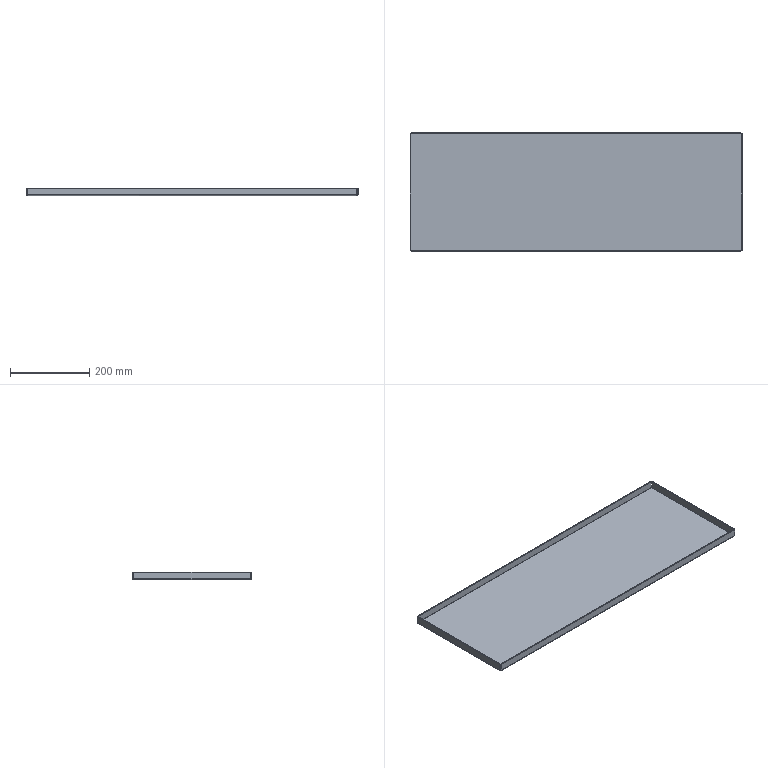Part | STEP file | Part 14 | 1 solid | 38 faces | box 840 x 300 x 20 mm | volume 582338 mm3 | plane 22 | spline 8 | cylinder 8 | commonest cylinder face diameters 1 x4 5 x4
STEP:
#1=CARTESIAN_POINT('',(-417.5,-147.5,-2.));
#2=VERTEX_POINT('',#1);
#3=CARTESIAN_POINT('',(-417.5,147.5,-2.));
#4=VERTEX_POINT('',#3);
#5=CARTESIAN_POINT('',(-417.5,-147.5,-2.));
#6=DIRECTION('',(0.,1.,0.));
#7=VECTOR('',#6,1000.);
#8=LINE('',#5,#7);
#9=EDGE_CURVE('',#2,#4,#8,.T.);
#10=ORIENTED_EDGE('',*,*,#9,.T.);
#11=CARTESIAN_POINT('',(417.5,147.5,-2.));
#12=VERTEX_POINT('',#11);
#13=CARTESIAN_POINT('',(-417.5,147.5,-2.));
#14=DIRECTION('',(1.,0.,0.));
#15=VECTOR('',#14,1000.);
#16=LINE('',#13,#15);
#17=EDGE_CURVE('',#4,#12,#16,.T.);
#18=ORIENTED_EDGE('',*,*,#17,.T.);
#19=CARTESIAN_POINT('',(417.5,-147.5,-2.));
#20=VERTEX_POINT('',#19);
#21=CARTESIAN_POINT('',(417.5,147.5,-2.));
#22=DIRECTION('',(0.,-1.,0.));
#23=VECTOR('',#22,1000.);
#24=LINE('',#21,#23);
#25=EDGE_CURVE('',#12,#20,#24,.T.);
#26=ORIENTED_EDGE('',*,*,#25,.T.);
#27=CARTESIAN_POINT('',(417.5,-147.5,-2.));
#28=DIRECTION('',(-1.,0.,0.));
#29=VECTOR('',#28,1000.);
#30=LINE('',#27,#29);
#31=EDGE_CURVE('',#20,#2,#30,.T.);
#32=ORIENTED_EDGE('',*,*,#31,.T.);
#33=EDGE_LOOP('',(#10,#18,#26,#32));
#34=FACE_OUTER_BOUND('',#33,.T.);
#35=CARTESIAN_POINT('',(0.,0.,-2.));
#36=DIRECTION('',(0.,0.,1.));
#37=DIRECTION('',(1.,0.,0.));
#38=AXIS2_PLACEMENT_3D('',#35,#36,#37);
#39=PLANE('',#38);
#40=ADVANCED_FACE('',(#34),#39,.F.);
#41=CARTESIAN_POINT('',(-417.5,147.5,0.));
#42=VERTEX_POINT('',#41);
#43=CARTESIAN_POINT('',(417.5,147.5,0.));
#44=VERTEX_POINT('',#43);
#45=CARTESIAN_POINT('',(-417.5,147.5,0.));
#46=DIRECTION('',(1.,0.,0.));
#47=VECTOR('',#46,1000.);
#48=LINE('',#45,#47);
#49=EDGE_CURVE('',#42,#44,#48,.T.);
#50=ORIENTED_EDGE('',*,*,#49,.F.);
#51=CARTESIAN_POINT('',(-417.5,-147.5,0.));
#52=VERTEX_POINT('',#51);
#53=CARTESIAN_POINT('',(-417.5,-147.5,0.));
#54=DIRECTION('',(0.,1.,0.));
#55=VECTOR('',#54,1000.);
#56=LINE('',#53,#55);
#57=EDGE_CURVE('',#52,#42,#56,.T.);
#58=ORIENTED_EDGE('',*,*,#57,.F.);
#59=CARTESIAN_POINT('',(417.5,-147.5,0.));
#60=VERTEX_POINT('',#59);
#61=CARTESIAN_POINT('',(417.5,-147.5,0.));
#62=DIRECTION('',(-1.,0.,0.));
#63=VECTOR('',#62,1000.);
#64=LINE('',#61,#63);
#65=EDGE_CURVE('',#60,#52,#64,.T.);
#66=ORIENTED_EDGE('',*,*,#65,.F.);
#67=CARTESIAN_POINT('',(417.5,147.5,0.));
#68=DIRECTION('',(0.,-1.,0.));
#69=VECTOR('',#68,1000.);
#70=LINE('',#67,#69);
#71=EDGE_CURVE('',#44,#60,#70,.T.);
#72=ORIENTED_EDGE('',*,*,#71,.F.);
#73=EDGE_LOOP('',(#50,#58,#66,#72));
#74=FACE_OUTER_BOUND('',#73,.T.);
#75=CARTESIAN_POINT('',(0.,0.,0.));
#76=DIRECTION('',(0.,0.,1.));
#77=DIRECTION('',(1.,0.,0.));
#78=AXIS2_PLACEMENT_3D('',#75,#76,#77);
#79=PLANE('',#78);
#80=ADVANCED_FACE('',(#74),#79,.T.);
#81=CARTESIAN_POINT('',(417.293,150.,0.5));
#82=VERTEX_POINT('',#81);
#83=CARTESIAN_POINT('',(417.293,148.,0.5));
#84=VERTEX_POINT('',#83);
#85=CARTESIAN_POINT('',(417.293,148.,0.5));
#86=DIRECTION('',(0.,-1.,0.));
#87=VECTOR('',#86,1000.);
#88=LINE('',#85,#87);
#89=EDGE_CURVE('',#82,#84,#88,.T.);
#90=ORIENTED_EDGE('',*,*,#89,.T.);
#91=CARTESIAN_POINT('',(417.5,147.5,0.));
#92=CARTESIAN_POINT('',(417.465,147.631,0.));
#93=CARTESIAN_POINT('',(417.431,147.761,0.05389));
#94=CARTESIAN_POINT('',(417.362,147.946,0.239));
#95=CARTESIAN_POINT('',(417.327,148.,0.3691));
#96=CARTESIAN_POINT('',(417.293,148.,0.5));
#97=B_SPLINE_CURVE_WITH_KNOTS('',3,(#91,#92,#93,#94,#95,#96),.UNSPECIFIED.,.F.,.F.,(4,2,4),(0.,0.5,1.),.UNSPECIFIED.);
#98=EDGE_CURVE('',#44,#84,#97,.T.);
#99=ORIENTED_EDGE('',*,*,#98,.F.);
#100=CARTESIAN_POINT('',(417.5,147.5,0.));
#101=DIRECTION('',(0.,0.,-1.));
#102=VECTOR('',#101,1000.);
#103=LINE('',#100,#102);
#104=EDGE_CURVE('',#44,#12,#103,.T.);
#105=ORIENTED_EDGE('',*,*,#104,.T.);
#106=CARTESIAN_POINT('',(417.5,147.5,-2.));
#107=CARTESIAN_POINT('',(417.483,147.827,-2.));
#108=CARTESIAN_POINT('',(417.465,148.154,-1.935));
#109=CARTESIAN_POINT('',(417.431,148.759,-1.684));
#110=CARTESIAN_POINT('',(417.414,149.036,-1.499));
#111=CARTESIAN_POINT('',(417.379,149.499,-1.036));
#112=CARTESIAN_POINT('',(417.362,149.684,-0.759));
#113=CARTESIAN_POINT('',(417.327,149.935,-0.1544));
#114=CARTESIAN_POINT('',(417.31,150.,0.1728));
#115=CARTESIAN_POINT('',(417.293,150.,0.5));
#116=B_SPLINE_CURVE_WITH_KNOTS('',3,(#106,#107,#108,#109,#110,#111,#112,#113,#114,#115),.UNSPECIFIED.,.F.,.F.,(4,2,2,2,4),(0.,0.25,0.5,0.75,1.),.UNSPECIFIED.);
#117=EDGE_CURVE('',#12,#82,#116,.T.);
#118=ORIENTED_EDGE('',*,*,#117,.T.);
#119=EDGE_LOOP('',(#90,#99,#105,#118));
#120=FACE_OUTER_BOUND('',#119,.T.);
#121=CARTESIAN_POINT('',(417.5,147.5,-2.02));
#122=CARTESIAN_POINT('',(417.483,147.83,-2.02));
#123=CARTESIAN_POINT('',(417.465,148.16,-1.954));
#124=CARTESIAN_POINT('',(417.431,148.769,-1.702));
#125=CARTESIAN_POINT('',(417.414,149.049,-1.515));
#126=CARTESIAN_POINT('',(417.379,149.515,-1.049));
#127=CARTESIAN_POINT('',(417.362,149.702,-0.7691));
#128=CARTESIAN_POINT('',(417.327,149.954,-0.1596));
#129=CARTESIAN_POINT('',(417.31,150.02,0.1701));
#130=CARTESIAN_POINT('',(417.293,150.02,0.5));
#131=CARTESIAN_POINT('',(417.5,147.5,-2.));
#132=CARTESIAN_POINT('',(417.483,147.827,-2.));
#133=CARTESIAN_POINT('',(417.465,148.154,-1.935));
#134=CARTESIAN_POINT('',(417.431,148.759,-1.684));
#135=CARTESIAN_POINT('',(417.414,149.036,-1.499));
#136=CARTESIAN_POINT('',(417.379,149.499,-1.036));
#137=CARTESIAN_POINT('',(417.362,149.684,-0.759));
#138=CARTESIAN_POINT('',(417.327,149.935,-0.1544));
#139=CARTESIAN_POINT('',(417.31,150.,0.1727));
#140=CARTESIAN_POINT('',(417.293,150.,0.5));
#141=CARTESIAN_POINT('',(417.5,147.5,0.));
#142=CARTESIAN_POINT('',(417.483,147.565,0.));
#143=CARTESIAN_POINT('',(417.465,147.631,0.01301));
#144=CARTESIAN_POINT('',(417.431,147.752,0.06311));
#145=CARTESIAN_POINT('',(417.414,147.807,0.1002));
#146=CARTESIAN_POINT('',(417.379,147.9,0.1927));
#147=CARTESIAN_POINT('',(417.362,147.937,0.2482));
#148=CARTESIAN_POINT('',(417.327,147.987,0.3691));
#149=CARTESIAN_POINT('',(417.31,148.,0.4345));
#150=CARTESIAN_POINT('',(417.293,148.,0.5));
#151=CARTESIAN_POINT('',(417.5,147.5,0.0202));
#152=CARTESIAN_POINT('',(417.483,147.563,0.0202));
#153=CARTESIAN_POINT('',(417.465,147.626,0.03269));
#154=CARTESIAN_POINT('',(417.431,147.742,0.08076));
#155=CARTESIAN_POINT('',(417.414,147.795,0.1163));
#156=CARTESIAN_POINT('',(417.379,147.884,0.2051));
#157=CARTESIAN_POINT('',(417.362,147.919,0.2584));
#158=CARTESIAN_POINT('',(417.327,147.967,0.3744));
#159=CARTESIAN_POINT('',(417.31,147.98,0.4372));
#160=CARTESIAN_POINT('',(417.293,147.98,0.5));
#161=B_SPLINE_SURFACE_WITH_KNOTS('',1,3,((#121,#122,#123,#124,#125,#126,#127,#128,#129,#130),(#131,#132,#133,#134,#135,#136,#137,#138,#139,#140),(#141,#142,#143,#144,#145,#146,#147,#148,#149,#150),(#151,#152,#153,#154,#155,#156,#157,#158,#159,#160)),.UNSPECIFIED.,.F.,.F.,.F.,(2,1,1,2),(4,2,2,2,4),(-0.01,0.,1.,1.01),(0.,0.25,0.5,0.75,1.),.UNSPECIFIED.);
#162=ADVANCED_FACE('',(#120),#161,.F.);
#163=CARTESIAN_POINT('',(-417.293,148.,0.5));
#164=VERTEX_POINT('',#163);
#165=CARTESIAN_POINT('',(-417.293,148.,0.5));
#166=CARTESIAN_POINT('',(-417.327,148.,0.3691));
#167=CARTESIAN_POINT('',(-417.362,147.946,0.239));
#168=CARTESIAN_POINT('',(-417.431,147.761,0.05389));
#169=CARTESIAN_POINT('',(-417.465,147.631,0.));
#170=CARTESIAN_POINT('',(-417.5,147.5,0.));
#171=B_SPLINE_CURVE_WITH_KNOTS('',3,(#165,#166,#167,#168,#169,#170),.UNSPECIFIED.,.F.,.F.,(4,2,4),(0.,0.5,1.),.UNSPECIFIED.);
#172=EDGE_CURVE('',#164,#42,#171,.T.);
#173=ORIENTED_EDGE('',*,*,#172,.F.);
#174=CARTESIAN_POINT('',(-417.293,150.,0.5));
#175=VERTEX_POINT('',#174);
#176=CARTESIAN_POINT('',(-417.293,148.,0.5));
#177=DIRECTION('',(0.,-1.,0.));
#178=VECTOR('',#177,1000.);
#179=LINE('',#176,#178);
#180=EDGE_CURVE('',#175,#164,#179,.T.);
#181=ORIENTED_EDGE('',*,*,#180,.F.);
#182=CARTESIAN_POINT('',(-417.293,150.,0.5));
#183=CARTESIAN_POINT('',(-417.31,150.,0.1728));
#184=CARTESIAN_POINT('',(-417.327,149.935,-0.1544));
#185=CARTESIAN_POINT('',(-417.362,149.684,-0.759));
#186=CARTESIAN_POINT('',(-417.379,149.499,-1.036));
#187=CARTESIAN_POINT('',(-417.414,149.036,-1.499));
#188=CARTESIAN_POINT('',(-417.431,148.759,-1.684));
#189=CARTESIAN_POINT('',(-417.465,148.154,-1.935));
#190=CARTESIAN_POINT('',(-417.483,147.827,-2.));
#191=CARTESIAN_POINT('',(-417.5,147.5,-2.));
#192=B_SPLINE_CURVE_WITH_KNOTS('',3,(#182,#183,#184,#185,#186,#187,#188,#189,#190,#191),.UNSPECIFIED.,.F.,.F.,(4,2,2,2,4),(0.,0.25,0.5,0.75,1.),.UNSPECIFIED.);
#193=EDGE_CURVE('',#175,#4,#192,.T.);
#194=ORIENTED_EDGE('',*,*,#193,.T.);
#195=CARTESIAN_POINT('',(-417.5,147.5,0.));
#196=DIRECTION('',(0.,0.,-1.));
#197=VECTOR('',#196,1000.);
#198=LINE('',#195,#197);
#199=EDGE_CURVE('',#42,#4,#198,.T.);
#200=ORIENTED_EDGE('',*,*,#199,.F.);
#201=EDGE_LOOP('',(#173,#181,#194,#200));
#202=FACE_OUTER_BOUND('',#201,.T.);
#203=CARTESIAN_POINT('',(-417.293,150.02,0.5));
#204=CARTESIAN_POINT('',(-417.31,150.02,0.1701));
#205=CARTESIAN_POINT('',(-417.327,149.954,-0.1596));
#206=CARTESIAN_POINT('',(-417.362,149.702,-0.7691));
#207=CARTESIAN_POINT('',(-417.379,149.515,-1.049));
#208=CARTESIAN_POINT('',(-417.414,149.049,-1.515));
#209=CARTESIAN_POINT('',(-417.431,148.769,-1.702));
#210=CARTESIAN_POINT('',(-417.465,148.16,-1.954));
#211=CARTESIAN_POINT('',(-417.483,147.83,-2.02));
#212=CARTESIAN_POINT('',(-417.5,147.5,-2.02));
#213=CARTESIAN_POINT('',(-417.293,150.,0.5));
#214=CARTESIAN_POINT('',(-417.31,150.,0.1727));
#215=CARTESIAN_POINT('',(-417.327,149.935,-0.1544));
#216=CARTESIAN_POINT('',(-417.362,149.684,-0.759));
#217=CARTESIAN_POINT('',(-417.379,149.499,-1.036));
#218=CARTESIAN_POINT('',(-417.414,149.036,-1.499));
#219=CARTESIAN_POINT('',(-417.431,148.759,-1.684));
#220=CARTESIAN_POINT('',(-417.465,148.154,-1.935));
#221=CARTESIAN_POINT('',(-417.483,147.827,-2.));
#222=CARTESIAN_POINT('',(-417.5,147.5,-2.));
#223=CARTESIAN_POINT('',(-417.293,148.,0.5));
#224=CARTESIAN_POINT('',(-417.31,148.,0.4345));
#225=CARTESIAN_POINT('',(-417.327,147.987,0.3691));
#226=CARTESIAN_POINT('',(-417.362,147.937,0.2482));
#227=CARTESIAN_POINT('',(-417.379,147.9,0.1927));
#228=CARTESIAN_POINT('',(-417.414,147.807,0.1002));
#229=CARTESIAN_POINT('',(-417.431,147.752,0.06311));
#230=CARTESIAN_POINT('',(-417.465,147.631,0.01301));
#231=CARTESIAN_POINT('',(-417.483,147.565,0.));
#232=CARTESIAN_POINT('',(-417.5,147.5,0.));
#233=CARTESIAN_POINT('',(-417.293,147.98,0.5));
#234=CARTESIAN_POINT('',(-417.31,147.98,0.4372));
#235=CARTESIAN_POINT('',(-417.327,147.967,0.3744));
#236=CARTESIAN_POINT('',(-417.362,147.919,0.2584));
#237=CARTESIAN_POINT('',(-417.379,147.884,0.2051));
#238=CARTESIAN_POINT('',(-417.414,147.795,0.1163));
#239=CARTESIAN_POINT('',(-417.431,147.742,0.08076));
#240=CARTESIAN_POINT('',(-417.465,147.626,0.03269));
#241=CARTESIAN_POINT('',(-417.483,147.563,0.0202));
#242=CARTESIAN_POINT('',(-417.5,147.5,0.0202));
#243=B_SPLINE_SURFACE_WITH_KNOTS('',1,3,((#203,#204,#205,#206,#207,#208,#209,#210,#211,#212),(#213,#214,#215,#216,#217,#218,#219,#220,#221,#222),(#223,#224,#225,#226,#227,#228,#229,#230,#231,#232),(#233,#234,#235,#236,#237,#238,#239,#240,#241,#242)),.UNSPECIFIED.,.F.,.F.,.F.,(2,1,1,2),(4,2,2,2,4),(-0.01,0.,1.,1.01),(0.,0.25,0.5,0.75,1.),.UNSPECIFIED.);
#244=ADVANCED_FACE('',(#202),#243,.F.);
#245=ORIENTED_EDGE('',*,*,#17,.F.);
#246=ORIENTED_EDGE('',*,*,#193,.F.);
#247=CARTESIAN_POINT('',(0.,150.,0.5));
#248=DIRECTION('',(-1.,0.,0.));
#249=VECTOR('',#248,1000.);
#250=LINE('',#247,#249);
#251=EDGE_CURVE('',#82,#175,#250,.T.);
#252=ORIENTED_EDGE('',*,*,#251,.F.);
#253=ORIENTED_EDGE('',*,*,#117,.F.);
#254=EDGE_LOOP('',(#245,#246,#252,#253));
#255=FACE_OUTER_BOUND('',#254,.T.);
#256=CARTESIAN_POINT('',(-417.5,147.5,0.5));
#257=DIRECTION('',(-1.,0.,0.));
#258=DIRECTION('',(0.,1.,0.));
#259=AXIS2_PLACEMENT_3D('',#256,#257,#258);
#260=CYLINDRICAL_SURFACE('',#259,2.5);
#261=ADVANCED_FACE('',(#255),#260,.T.);
#262=ORIENTED_EDGE('',*,*,#49,.T.);
#263=ORIENTED_EDGE('',*,*,#98,.T.);
#264=CARTESIAN_POINT('',(420.,148.,0.5));
#265=DIRECTION('',(-1.,0.,0.));
#266=VECTOR('',#265,1000.);
#267=LINE('',#264,#266);
#268=EDGE_CURVE('',#84,#164,#267,.T.);
#269=ORIENTED_EDGE('',*,*,#268,.T.);
#270=ORIENTED_EDGE('',*,*,#172,.T.);
#271=EDGE_LOOP('',(#262,#263,#269,#270));
#272=FACE_OUTER_BOUND('',#271,.T.);
#273=CARTESIAN_POINT('',(-417.5,147.5,0.5));
#274=DIRECTION('',(-1.,0.,0.));
#275=DIRECTION('',(0.,1.,0.));
#276=AXIS2_PLACEMENT_3D('',#273,#274,#275);
#277=CYLINDRICAL_SURFACE('',#276,0.5);
#278=ADVANCED_FACE('',(#272),#277,.F.);
#279=CARTESIAN_POINT('',(417.293,148.,18.));
#280=VERTEX_POINT('',#279);
#281=CARTESIAN_POINT('',(417.293,150.,18.));
#282=VERTEX_POINT('',#281);
#283=CARTESIAN_POINT('',(417.293,150.,18.));
#284=DIRECTION('',(0.,1.,0.));
#285=VECTOR('',#284,1000.);
#286=LINE('',#283,#285);
#287=EDGE_CURVE('',#280,#282,#286,.T.);
#288=ORIENTED_EDGE('',*,*,#287,.F.);
#289=CARTESIAN_POINT('',(417.293,148.,0.));
#290=DIRECTION('',(0.,0.,1.));
#291=VECTOR('',#290,1000.);
#292=LINE('',#289,#291);
#293=EDGE_CURVE('',#84,#280,#292,.T.);
#294=ORIENTED_EDGE('',*,*,#293,.F.);
#295=ORIENTED_EDGE('',*,*,#89,.F.);
#296=CARTESIAN_POINT('',(417.293,150.,0.));
#297=DIRECTION('',(0.,0.,-1.));
#298=VECTOR('',#297,1000.);
#299=LINE('',#296,#298);
#300=EDGE_CURVE('',#282,#82,#299,.T.);
#301=ORIENTED_EDGE('',*,*,#300,.F.);
#302=EDGE_LOOP('',(#288,#294,#295,#301));
#303=FACE_OUTER_BOUND('',#302,.T.);
#304=CARTESIAN_POINT('',(417.293,148.,0.));
#305=DIRECTION('',(1.,0.,0.));
#306=DIRECTION('',(0.,0.,-1.));
#307=AXIS2_PLACEMENT_3D('',#304,#305,#306);
#308=PLANE('',#307);
#309=ADVANCED_FACE('',(#303),#308,.T.);
#310=CARTESIAN_POINT('',(-417.293,150.,18.));
#311=VERTEX_POINT('',#310);
#312=CARTESIAN_POINT('',(-417.293,150.,0.));
#313=DIRECTION('',(0.,0.,-1.));
#314=VECTOR('',#313,1000.);
#315=LINE('',#312,#314);
#316=EDGE_CURVE('',#311,#175,#315,.T.);
#317=ORIENTED_EDGE('',*,*,#316,.F.);
#318=CARTESIAN_POINT('',(-420.,150.,18.));
#319=DIRECTION('',(-1.,0.,0.));
#320=VECTOR('',#319,1000.);
#321=LINE('',#318,#320);
#322=EDGE_CURVE('',#282,#311,#321,.T.);
#323=ORIENTED_EDGE('',*,*,#322,.F.);
#324=ORIENTED_EDGE('',*,*,#300,.T.);
#325=ORIENTED_EDGE('',*,*,#251,.T.);
#326=EDGE_LOOP('',(#317,#323,#324,#325));
#327=FACE_OUTER_BOUND('',#326,.T.);
#328=CARTESIAN_POINT('',(0.,150.,0.));
#329=DIRECTION('',(0.,1.,0.));
#330=DIRECTION('',(0.,0.,1.));
#331=AXIS2_PLACEMENT_3D('',#328,#329,#330);
#332=PLANE('',#331);
#333=ADVANCED_FACE('',(#327),#332,.T.);
#334=CARTESIAN_POINT('',(-417.293,148.,18.));
#335=VERTEX_POINT('',#334);
#336=CARTESIAN_POINT('',(0.,148.,18.));
#337=DIRECTION('',(-1.,0.,0.));
#338=VECTOR('',#337,1000.);
#339=LINE('',#336,#338);
#340=EDGE_CURVE('',#280,#335,#339,.T.);
#341=ORIENTED_EDGE('',*,*,#340,.T.);
#342=CARTESIAN_POINT('',(-417.293,148.,0.));
#343=DIRECTION('',(0.,0.,1.));
#344=VECTOR('',#343,1000.);
#345=LINE('',#342,#344);
#346=EDGE_CURVE('',#164,#335,#345,.T.);
#347=ORIENTED_EDGE('',*,*,#346,.F.);
#348=ORIENTED_EDGE('',*,*,#268,.F.);
#349=ORIENTED_EDGE('',*,*,#293,.T.);
#350=EDGE_LOOP('',(#341,#347,#348,#349));
#351=FACE_OUTER_BOUND('',#350,.T.);
#352=CARTESIAN_POINT('',(0.,148.,0.));
#353=DIRECTION('',(0.,1.,0.));
#354=DIRECTION('',(0.,0.,1.));
#355=AXIS2_PLACEMENT_3D('',#352,#353,#354);
#356=PLANE('',#355);
#357=ADVANCED_FACE('',(#351),#356,.F.);
#358=CARTESIAN_POINT('',(-417.293,148.,18.));
#359=DIRECTION('',(0.,1.,0.));
#360=VECTOR('',#359,1000.);
#361=LINE('',#358,#360);
#362=EDGE_CURVE('',#335,#311,#361,.T.);
#363=ORIENTED_EDGE('',*,*,#362,.F.);
#364=ORIENTED_EDGE('',*,*,#340,.F.);
#365=ORIENTED_EDGE('',*,*,#287,.T.);
#366=ORIENTED_EDGE('',*,*,#322,.T.);
#367=EDGE_LOOP('',(#363,#364,#365,#366));
#368=FACE_OUTER_BOUND('',#367,.T.);
#369=CARTESIAN_POINT('',(-420.,150.,18.));
#370=DIRECTION('',(0.,0.,1.));
#371=DIRECTION('',(0.,-1.,0.));
#372=AXIS2_PLACEMENT_3D('',#369,#370,#371);
#373=PLANE('',#372);
#374=ADVANCED_FACE('',(#368),#373,.T.);
#375=ORIENTED_EDGE('',*,*,#346,.T.);
#376=ORIENTED_EDGE('',*,*,#362,.T.);
#377=ORIENTED_EDGE('',*,*,#316,.T.);
#378=ORIENTED_EDGE('',*,*,#180,.T.);
#379=EDGE_LOOP('',(#375,#376,#377,#378));
#380=FACE_OUTER_BOUND('',#379,.T.);
#381=CARTESIAN_POINT('',(-417.293,148.,0.));
#382=DIRECTION('',(1.,0.,0.));
#383=DIRECTION('',(0.,0.,-1.));
#384=AXIS2_PLACEMENT_3D('',#381,#382,#383);
#385=PLANE('',#384);
#386=ADVANCED_FACE('',(#380),#385,.F.);
#387=CARTESIAN_POINT('',(420.,-147.293,0.5));
#388=VERTEX_POINT('',#387);
#389=CARTESIAN_POINT('',(418.,-147.293,0.5));
#390=VERTEX_POINT('',#389);
#391=CARTESIAN_POINT('',(418.,-147.293,0.5));
#392=DIRECTION('',(-1.,0.,0.));
#393=VECTOR('',#392,1000.);
#394=LINE('',#391,#393);
#395=EDGE_CURVE('',#388,#390,#394,.T.);
#396=ORIENTED_EDGE('',*,*,#395,.T.);
#397=CARTESIAN_POINT('',(417.5,-147.5,0.));
#398=CARTESIAN_POINT('',(417.631,-147.465,0.));
#399=CARTESIAN_POINT('',(417.761,-147.431,0.05389));
#400=CARTESIAN_POINT('',(417.946,-147.362,0.239));
#401=CARTESIAN_POINT('',(418.,-147.327,0.3691));
#402=CARTESIAN_POINT('',(418.,-147.293,0.5));
#403=B_SPLINE_CURVE_WITH_KNOTS('',3,(#397,#398,#399,#400,#401,#402),.UNSPECIFIED.,.F.,.F.,(4,2,4),(0.,0.5,1.),.UNSPECIFIED.);
#404=EDGE_CURVE('',#60,#390,#403,.T.);
#405=ORIENTED_EDGE('',*,*,#404,.F.);
#406=CARTESIAN_POINT('',(417.5,-147.5,0.));
#407=DIRECTION('',(0.,0.,-1.));
#408=VECTOR('',#407,1000.);
#409=LINE('',#406,#408);
#410=EDGE_CURVE('',#60,#20,#409,.T.);
#411=ORIENTED_EDGE('',*,*,#410,.T.);
#412=CARTESIAN_POINT('',(417.5,-147.5,-2.));
#413=CARTESIAN_POINT('',(417.827,-147.483,-2.));
#414=CARTESIAN_POINT('',(418.154,-147.465,-1.935));
#415=CARTESIAN_POINT('',(418.759,-147.431,-1.684));
#416=CARTESIAN_POINT('',(419.036,-147.414,-1.499));
#417=CARTESIAN_POINT('',(419.499,-147.379,-1.036));
#418=CARTESIAN_POINT('',(419.684,-147.362,-0.759));
#419=CARTESIAN_POINT('',(419.935,-147.327,-0.1544));
#420=CARTESIAN_POINT('',(420.,-147.31,0.1728));
#421=CARTESIAN_POINT('',(420.,-147.293,0.5));
#422=B_SPLINE_CURVE_WITH_KNOTS('',3,(#412,#413,#414,#415,#416,#417,#418,#419,#420,#421),.UNSPECIFIED.,.F.,.F.,(4,2,2,2,4),(0.,0.25,0.5,0.75,1.),.UNSPECIFIED.);
#423=EDGE_CURVE('',#20,#388,#422,.T.);
#424=ORIENTED_EDGE('',*,*,#423,.T.);
#425=EDGE_LOOP('',(#396,#405,#411,#424));
#426=FACE_OUTER_BOUND('',#425,.T.);
#427=CARTESIAN_POINT('',(417.5,-147.5,-2.02));
#428=CARTESIAN_POINT('',(417.83,-147.483,-2.02));
#429=CARTESIAN_POINT('',(418.16,-147.465,-1.954));
#430=CARTESIAN_POINT('',(418.769,-147.431,-1.702));
#431=CARTESIAN_POINT('',(419.049,-147.414,-1.515));
#432=CARTESIAN_POINT('',(419.515,-147.379,-1.049));
#433=CARTESIAN_POINT('',(419.702,-147.362,-0.7691));
#434=CARTESIAN_POINT('',(419.954,-147.327,-0.1596));
#435=CARTESIAN_POINT('',(420.02,-147.31,0.1701));
#436=CARTESIAN_POINT('',(420.02,-147.293,0.5));
#437=CARTESIAN_POINT('',(417.5,-147.5,-2.));
#438=CARTESIAN_POINT('',(417.827,-147.483,-2.));
#439=CARTESIAN_POINT('',(418.154,-147.465,-1.935));
#440=CARTESIAN_POINT('',(418.759,-147.431,-1.684));
#441=CARTESIAN_POINT('',(419.036,-147.414,-1.499));
#442=CARTESIAN_POINT('',(419.499,-147.379,-1.036));
#443=CARTESIAN_POINT('',(419.684,-147.362,-0.759));
#444=CARTESIAN_POINT('',(419.935,-147.327,-0.1544));
#445=CARTESIAN_POINT('',(420.,-147.31,0.1727));
#446=CARTESIAN_POINT('',(420.,-147.293,0.5));
#447=CARTESIAN_POINT('',(417.5,-147.5,0.));
#448=CARTESIAN_POINT('',(417.565,-147.483,0.));
#449=CARTESIAN_POINT('',(417.631,-147.465,0.01301));
#450=CARTESIAN_POINT('',(417.752,-147.431,0.06311));
#451=CARTESIAN_POINT('',(417.807,-147.414,0.1002));
#452=CARTESIAN_POINT('',(417.9,-147.379,0.1927));
#453=CARTESIAN_POINT('',(417.937,-147.362,0.2482));
#454=CARTESIAN_POINT('',(417.987,-147.327,0.3691));
#455=CARTESIAN_POINT('',(418.,-147.31,0.4345));
#456=CARTESIAN_POINT('',(418.,-147.293,0.5));
#457=CARTESIAN_POINT('',(417.5,-147.5,0.0202));
#458=CARTESIAN_POINT('',(417.563,-147.483,0.0202));
#459=CARTESIAN_POINT('',(417.626,-147.465,0.03269));
#460=CARTESIAN_POINT('',(417.742,-147.431,0.08076));
#461=CARTESIAN_POINT('',(417.795,-147.414,0.1163));
#462=CARTESIAN_POINT('',(417.884,-147.379,0.2051));
#463=CARTESIAN_POINT('',(417.919,-147.362,0.2584));
#464=CARTESIAN_POINT('',(417.967,-147.327,0.3744));
#465=CARTESIAN_POINT('',(417.98,-147.31,0.4372));
#466=CARTESIAN_POINT('',(417.98,-147.293,0.5));
#467=B_SPLINE_SURFACE_WITH_KNOTS('',1,3,((#427,#428,#429,#430,#431,#432,#433,#434,#435,#436),(#437,#438,#439,#440,#441,#442,#443,#444,#445,#446),(#447,#448,#449,#450,#451,#452,#453,#454,#455,#456),(#457,#458,#459,#460,#461,#462,#463,#464,#465,#466)),.UNSPECIFIED.,.F.,.F.,.F.,(2,1,1,2),(4,2,2,2,4),(-0.01,0.,1.,1.01),(0.,0.25,0.5,0.75,1.),.UNSPECIFIED.);
#468=ADVANCED_FACE('',(#426),#467,.F.);
#469=CARTESIAN_POINT('',(418.,147.293,0.5));
#470=VERTEX_POINT('',#469);
#471=CARTESIAN_POINT('',(418.,147.293,0.5));
#472=CARTESIAN_POINT('',(418.,147.327,0.3691));
#473=CARTESIAN_POINT('',(417.946,147.362,0.239));
#474=CARTESIAN_POINT('',(417.761,147.431,0.05389));
#475=CARTESIAN_POINT('',(417.631,147.465,0.));
#476=CARTESIAN_POINT('',(417.5,147.5,0.));
#477=B_SPLINE_CURVE_WITH_KNOTS('',3,(#471,#472,#473,#474,#475,#476),.UNSPECIFIED.,.F.,.F.,(4,2,4),(0.,0.5,1.),.UNSPECIFIED.);
#478=EDGE_CURVE('',#470,#44,#477,.T.);
#479=ORIENTED_EDGE('',*,*,#478,.F.);
#480=CARTESIAN_POINT('',(420.,147.293,0.5));
#481=VERTEX_POINT('',#480);
#482=CARTESIAN_POINT('',(418.,147.293,0.5));
#483=DIRECTION('',(-1.,0.,0.));
#484=VECTOR('',#483,1000.);
#485=LINE('',#482,#484);
#486=EDGE_CURVE('',#481,#470,#485,.T.);
#487=ORIENTED_EDGE('',*,*,#486,.F.);
#488=CARTESIAN_POINT('',(420.,147.293,0.5));
#489=CARTESIAN_POINT('',(420.,147.31,0.1728));
#490=CARTESIAN_POINT('',(419.935,147.327,-0.1544));
#491=CARTESIAN_POINT('',(419.684,147.362,-0.759));
#492=CARTESIAN_POINT('',(419.499,147.379,-1.036));
#493=CARTESIAN_POINT('',(419.036,147.414,-1.499));
#494=CARTESIAN_POINT('',(418.759,147.431,-1.684));
#495=CARTESIAN_POINT('',(418.154,147.465,-1.935));
#496=CARTESIAN_POINT('',(417.827,147.483,-2.));
#497=CARTESIAN_POINT('',(417.5,147.5,-2.));
#498=B_SPLINE_CURVE_WITH_KNOTS('',3,(#488,#489,#490,#491,#492,#493,#494,#495,#496,#497),.UNSPECIFIED.,.F.,.F.,(4,2,2,2,4),(0.,0.25,0.5,0.75,1.),.UNSPECIFIED.);
#499=EDGE_CURVE('',#481,#12,#498,.T.);
#500=ORIENTED_EDGE('',*,*,#499,.T.);
#501=ORIENTED_EDGE('',*,*,#104,.F.);
#502=EDGE_LOOP('',(#479,#487,#500,#501));
#503=FACE_OUTER_BOUND('',#502,.T.);
#504=CARTESIAN_POINT('',(420.02,147.293,0.5));
#505=CARTESIAN_POINT('',(420.02,147.31,0.1701));
#506=CARTESIAN_POINT('',(419.954,147.327,-0.1596));
#507=CARTESIAN_POINT('',(419.702,147.362,-0.7691));
#508=CARTESIAN_POINT('',(419.515,147.379,-1.049));
#509=CARTESIAN_POINT('',(419.049,147.414,-1.515));
#510=CARTESIAN_POINT('',(418.769,147.431,-1.702));
#511=CARTESIAN_POINT('',(418.16,147.465,-1.954));
#512=CARTESIAN_POINT('',(417.83,147.483,-2.02));
#513=CARTESIAN_POINT('',(417.5,147.5,-2.02));
#514=CARTESIAN_POINT('',(420.,147.293,0.5));
#515=CARTESIAN_POINT('',(420.,147.31,0.1727));
#516=CARTESIAN_POINT('',(419.935,147.327,-0.1544));
#517=CARTESIAN_POINT('',(419.684,147.362,-0.759));
#518=CARTESIAN_POINT('',(419.499,147.379,-1.036));
#519=CARTESIAN_POINT('',(419.036,147.414,-1.499));
#520=CARTESIAN_POINT('',(418.759,147.431,-1.684));
#521=CARTESIAN_POINT('',(418.154,147.465,-1.935));
#522=CARTESIAN_POINT('',(417.827,147.483,-2.));
#523=CARTESIAN_POINT('',(417.5,147.5,-2.));
#524=CARTESIAN_POINT('',(418.,147.293,0.5));
#525=CARTESIAN_POINT('',(418.,147.31,0.4345));
#526=CARTESIAN_POINT('',(417.987,147.327,0.3691));
#527=CARTESIAN_POINT('',(417.937,147.362,0.2482));
#528=CARTESIAN_POINT('',(417.9,147.379,0.1927));
#529=CARTESIAN_POINT('',(417.807,147.414,0.1002));
#530=CARTESIAN_POINT('',(417.752,147.431,0.06311));
#531=CARTESIAN_POINT('',(417.631,147.465,0.01301));
#532=CARTESIAN_POINT('',(417.565,147.483,0.));
#533=CARTESIAN_POINT('',(417.5,147.5,0.));
#534=CARTESIAN_POINT('',(417.98,147.293,0.5));
#535=CARTESIAN_POINT('',(417.98,147.31,0.4372));
#536=CARTESIAN_POINT('',(417.967,147.327,0.3744));
#537=CARTESIAN_POINT('',(417.919,147.362,0.2584));
#538=CARTESIAN_POINT('',(417.884,147.379,0.2051));
#539=CARTESIAN_POINT('',(417.795,147.414,0.1163));
#540=CARTESIAN_POINT('',(417.742,147.431,0.08076));
#541=CARTESIAN_POINT('',(417.626,147.465,0.03269));
#542=CARTESIAN_POINT('',(417.563,147.483,0.0202));
#543=CARTESIAN_POINT('',(417.5,147.5,0.0202));
#544=B_SPLINE_SURFACE_WITH_KNOTS('',1,3,((#504,#505,#506,#507,#508,#509,#510,#511,#512,#513),(#514,#515,#516,#517,#518,#519,#520,#521,#522,#523),(#524,#525,#526,#527,#528,#529,#530,#531,#532,#533),(#534,#535,#536,#537,#538,#539,#540,#541,#542,#543)),.UNSPECIFIED.,.F.,.F.,.F.,(2,1,1,2),(4,2,2,2,4),(-0.01,0.,1.,1.01),(0.,0.25,0.5,0.75,1.),.UNSPECIFIED.);
#545=ADVANCED_FACE('',(#503),#544,.F.);
#546=ORIENTED_EDGE('',*,*,#25,.F.);
#547=ORIENTED_EDGE('',*,*,#499,.F.);
#548=CARTESIAN_POINT('',(420.,-150.,0.5));
#549=DIRECTION('',(0.,-1.,0.));
#550=VECTOR('',#549,1000.);
#551=LINE('',#548,#550);
#552=EDGE_CURVE('',#481,#388,#551,.T.);
#553=ORIENTED_EDGE('',*,*,#552,.T.);
#554=ORIENTED_EDGE('',*,*,#423,.F.);
#555=EDGE_LOOP('',(#546,#547,#553,#554));
#556=FACE_OUTER_BOUND('',#555,.T.);
#557=CARTESIAN_POINT('',(417.5,147.5,0.5));
#558=DIRECTION('',(0.,1.,0.));
#559=DIRECTION('',(1.,0.,0.));
#560=AXIS2_PLACEMENT_3D('',#557,#558,#559);
#561=CYLINDRICAL_SURFACE('',#560,2.5);
#562=ADVANCED_FACE('',(#556),#561,.T.);
#563=ORIENTED_EDGE('',*,*,#71,.T.);
#564=ORIENTED_EDGE('',*,*,#404,.T.);
#565=CARTESIAN_POINT('',(418.,-150.,0.5));
#566=DIRECTION('',(0.,1.,0.));
#567=VECTOR('',#566,1000.);
#568=LINE('',#565,#567);
#569=EDGE_CURVE('',#390,#470,#568,.T.);
#570=ORIENTED_EDGE('',*,*,#569,.T.);
#571=ORIENTED_EDGE('',*,*,#478,.T.);
#572=EDGE_LOOP('',(#563,#564,#570,#571));
#573=FACE_OUTER_BOUND('',#572,.T.);
#574=CARTESIAN_POINT('',(417.5,147.5,0.5));
#575=DIRECTION('',(0.,1.,0.));
#576=DIRECTION('',(1.,0.,0.));
#577=AXIS2_PLACEMENT_3D('',#574,#575,#576);
#578=CYLINDRICAL_SURFACE('',#577,0.5);
#579=ADVANCED_FACE('',(#573),#578,.F.);
#580=CARTESIAN_POINT('',(418.,-147.293,18.));
#581=VERTEX_POINT('',#580);
#582=CARTESIAN_POINT('',(420.,-147.293,18.));
#583=VERTEX_POINT('',#582);
#584=CARTESIAN_POINT('',(420.,-147.293,18.));
#585=DIRECTION('',(1.,0.,0.));
#586=VECTOR('',#585,1000.);
#587=LINE('',#584,#586);
#588=EDGE_CURVE('',#581,#583,#587,.T.);
#589=ORIENTED_EDGE('',*,*,#588,.F.);
#590=CARTESIAN_POINT('',(418.,-147.293,0.));
#591=DIRECTION('',(0.,0.,1.));
#592=VECTOR('',#591,1000.);
#593=LINE('',#590,#592);
#594=EDGE_CURVE('',#390,#581,#593,.T.);
#595=ORIENTED_EDGE('',*,*,#594,.F.);
#596=ORIENTED_EDGE('',*,*,#395,.F.);
#597=CARTESIAN_POINT('',(420.,-147.293,0.));
#598=DIRECTION('',(0.,0.,1.));
#599=VECTOR('',#598,1000.);
#600=LINE('',#597,#599);
#601=EDGE_CURVE('',#388,#583,#600,.T.);
#602=ORIENTED_EDGE('',*,*,#601,.T.);
#603=EDGE_LOOP('',(#589,#595,#596,#602));
#604=FACE_OUTER_BOUND('',#603,.T.);
#605=CARTESIAN_POINT('',(418.,-147.293,0.));
#606=DIRECTION('',(0.,-1.,0.));
#607=DIRECTION('',(0.,0.,-1.));
#608=AXIS2_PLACEMENT_3D('',#605,#606,#607);
#609=PLANE('',#608);
#610=ADVANCED_FACE('',(#604),#609,.T.);
#611=ORIENTED_EDGE('',*,*,#552,.F.);
#612=CARTESIAN_POINT('',(420.,147.293,18.));
#613=VERTEX_POINT('',#612);
#614=CARTESIAN_POINT('',(420.,147.293,0.));
#615=DIRECTION('',(0.,0.,1.));
#616=VECTOR('',#615,1000.);
#617=LINE('',#614,#616);
#618=EDGE_CURVE('',#481,#613,#617,.T.);
#619=ORIENTED_EDGE('',*,*,#618,.T.);
#620=CARTESIAN_POINT('',(420.,-150.,18.));
#621=DIRECTION('',(0.,1.,0.));
#622=VECTOR('',#621,1000.);
#623=LINE('',#620,#622);
#624=EDGE_CURVE('',#583,#613,#623,.T.);
#625=ORIENTED_EDGE('',*,*,#624,.F.);
#626=ORIENTED_EDGE('',*,*,#601,.F.);
#627=EDGE_LOOP('',(#611,#619,#625,#626));
#628=FACE_OUTER_BOUND('',#627,.T.);
#629=CARTESIAN_POINT('',(420.,0.,0.));
#630=DIRECTION('',(-1.,0.,0.));
#631=DIRECTION('',(0.,0.,1.));
#632=AXIS2_PLACEMENT_3D('',#629,#630,#631);
#633=PLANE('',#632);
#634=ADVANCED_FACE('',(#628),#633,.F.);
#635=CARTESIAN_POINT('',(418.,147.293,18.));
#636=VERTEX_POINT('',#635);
#637=CARTESIAN_POINT('',(418.,147.293,0.));
#638=DIRECTION('',(0.,0.,1.));
#639=VECTOR('',#638,1000.);
#640=LINE('',#637,#639);
#641=EDGE_CURVE('',#470,#636,#640,.T.);
#642=ORIENTED_EDGE('',*,*,#641,.F.);
#643=ORIENTED_EDGE('',*,*,#569,.F.);
#644=ORIENTED_EDGE('',*,*,#594,.T.);
#645=CARTESIAN_POINT('',(418.,0.,18.));
#646=DIRECTION('',(0.,1.,0.));
#647=VECTOR('',#646,1000.);
#648=LINE('',#645,#647);
#649=EDGE_CURVE('',#581,#636,#648,.T.);
#650=ORIENTED_EDGE('',*,*,#649,.T.);
#651=EDGE_LOOP('',(#642,#643,#644,#650));
#652=FACE_OUTER_BOUND('',#651,.T.);
#653=CARTESIAN_POINT('',(418.,0.,0.));
#654=DIRECTION('',(-1.,0.,0.));
#655=DIRECTION('',(0.,0.,1.));
#656=AXIS2_PLACEMENT_3D('',#653,#654,#655);
#657=PLANE('',#656);
#658=ADVANCED_FACE('',(#652),#657,.T.);
#659=CARTESIAN_POINT('',(418.,147.293,18.));
#660=DIRECTION('',(1.,0.,0.));
#661=VECTOR('',#660,1000.);
#662=LINE('',#659,#661);
#663=EDGE_CURVE('',#636,#613,#662,.T.);
#664=ORIENTED_EDGE('',*,*,#663,.F.);
#665=ORIENTED_EDGE('',*,*,#649,.F.);
#666=ORIENTED_EDGE('',*,*,#588,.T.);
#667=ORIENTED_EDGE('',*,*,#624,.T.);
#668=EDGE_LOOP('',(#664,#665,#666,#667));
#669=FACE_OUTER_BOUND('',#668,.T.);
#670=CARTESIAN_POINT('',(420.,-150.,18.));
#671=DIRECTION('',(0.,0.,1.));
#672=DIRECTION('',(1.,0.,0.));
#673=AXIS2_PLACEMENT_3D('',#670,#671,#672);
#674=PLANE('',#673);
#675=ADVANCED_FACE('',(#669),#674,.T.);
#676=ORIENTED_EDGE('',*,*,#641,.T.);
#677=ORIENTED_EDGE('',*,*,#663,.T.);
#678=ORIENTED_EDGE('',*,*,#618,.F.);
#679=ORIENTED_EDGE('',*,*,#486,.T.);
#680=EDGE_LOOP('',(#676,#677,#678,#679));
#681=FACE_OUTER_BOUND('',#680,.T.);
#682=CARTESIAN_POINT('',(418.,147.293,0.));
#683=DIRECTION('',(0.,-1.,0.));
#684=DIRECTION('',(0.,0.,-1.));
#685=AXIS2_PLACEMENT_3D('',#682,#683,#684);
#686=PLANE('',#685);
#687=ADVANCED_FACE('',(#681),#686,.F.);
#688=CARTESIAN_POINT('',(-417.293,-150.,0.5));
#689=VERTEX_POINT('',#688);
#690=CARTESIAN_POINT('',(-417.293,-148.,0.5));
#691=VERTEX_POINT('',#690);
#692=CARTESIAN_POINT('',(-417.293,-148.,0.5));
#693=DIRECTION('',(0.,1.,0.));
#694=VECTOR('',#693,1000.);
#695=LINE('',#692,#694);
#696=EDGE_CURVE('',#689,#691,#695,.T.);
#697=ORIENTED_EDGE('',*,*,#696,.T.);
#698=CARTESIAN_POINT('',(-417.5,-147.5,0.));
#699=CARTESIAN_POINT('',(-417.465,-147.631,0.));
#700=CARTESIAN_POINT('',(-417.431,-147.761,0.05389));
#701=CARTESIAN_POINT('',(-417.362,-147.946,0.239));
#702=CARTESIAN_POINT('',(-417.327,-148.,0.3691));
#703=CARTESIAN_POINT('',(-417.293,-148.,0.5));
#704=B_SPLINE_CURVE_WITH_KNOTS('',3,(#698,#699,#700,#701,#702,#703),.UNSPECIFIED.,.F.,.F.,(4,2,4),(0.,0.5,1.),.UNSPECIFIED.);
#705=EDGE_CURVE('',#52,#691,#704,.T.);
#706=ORIENTED_EDGE('',*,*,#705,.F.);
#707=CARTESIAN_POINT('',(-417.5,-147.5,0.));
#708=DIRECTION('',(0.,0.,-1.));
#709=VECTOR('',#708,1000.);
#710=LINE('',#707,#709);
#711=EDGE_CURVE('',#52,#2,#710,.T.);
#712=ORIENTED_EDGE('',*,*,#711,.T.);
#713=CARTESIAN_POINT('',(-417.5,-147.5,-2.));
#714=CARTESIAN_POINT('',(-417.483,-147.827,-2.));
#715=CARTESIAN_POINT('',(-417.465,-148.154,-1.935));
#716=CARTESIAN_POINT('',(-417.431,-148.759,-1.684));
#717=CARTESIAN_POINT('',(-417.414,-149.036,-1.499));
#718=CARTESIAN_POINT('',(-417.379,-149.499,-1.036));
#719=CARTESIAN_POINT('',(-417.362,-149.684,-0.759));
#720=CARTESIAN_POINT('',(-417.327,-149.935,-0.1544));
#721=CARTESIAN_POINT('',(-417.31,-150.,0.1728));
#722=CARTESIAN_POINT('',(-417.293,-150.,0.5));
#723=B_SPLINE_CURVE_WITH_KNOTS('',3,(#713,#714,#715,#716,#717,#718,#719,#720,#721,#722),.UNSPECIFIED.,.F.,.F.,(4,2,2,2,4),(0.,0.25,0.5,0.75,1.),.UNSPECIFIED.);
#724=EDGE_CURVE('',#2,#689,#723,.T.);
#725=ORIENTED_EDGE('',*,*,#724,.T.);
#726=EDGE_LOOP('',(#697,#706,#712,#725));
#727=FACE_OUTER_BOUND('',#726,.T.);
#728=CARTESIAN_POINT('',(-417.5,-147.5,-2.02));
#729=CARTESIAN_POINT('',(-417.483,-147.83,-2.02));
#730=CARTESIAN_POINT('',(-417.465,-148.16,-1.954));
#731=CARTESIAN_POINT('',(-417.431,-148.769,-1.702));
#732=CARTESIAN_POINT('',(-417.414,-149.049,-1.515));
#733=CARTESIAN_POINT('',(-417.379,-149.515,-1.049));
#734=CARTESIAN_POINT('',(-417.362,-149.702,-0.7691));
#735=CARTESIAN_POINT('',(-417.327,-149.954,-0.1596));
#736=CARTESIAN_POINT('',(-417.31,-150.02,0.1701));
#737=CARTESIAN_POINT('',(-417.293,-150.02,0.5));
#738=CARTESIAN_POINT('',(-417.5,-147.5,-2.));
#739=CARTESIAN_POINT('',(-417.483,-147.827,-2.));
#740=CARTESIAN_POINT('',(-417.465,-148.154,-1.935));
#741=CARTESIAN_POINT('',(-417.431,-148.759,-1.684));
#742=CARTESIAN_POINT('',(-417.414,-149.036,-1.499));
#743=CARTESIAN_POINT('',(-417.379,-149.499,-1.036));
#744=CARTESIAN_POINT('',(-417.362,-149.684,-0.759));
#745=CARTESIAN_POINT('',(-417.327,-149.935,-0.1544));
#746=CARTESIAN_POINT('',(-417.31,-150.,0.1727));
#747=CARTESIAN_POINT('',(-417.293,-150.,0.5));
#748=CARTESIAN_POINT('',(-417.5,-147.5,0.));
#749=CARTESIAN_POINT('',(-417.483,-147.565,0.));
#750=CARTESIAN_POINT('',(-417.465,-147.631,0.01301));
#751=CARTESIAN_POINT('',(-417.431,-147.752,0.06311));
#752=CARTESIAN_POINT('',(-417.414,-147.807,0.1002));
#753=CARTESIAN_POINT('',(-417.379,-147.9,0.1927));
#754=CARTESIAN_POINT('',(-417.362,-147.937,0.2482));
#755=CARTESIAN_POINT('',(-417.327,-147.987,0.3691));
#756=CARTESIAN_POINT('',(-417.31,-148.,0.4345));
#757=CARTESIAN_POINT('',(-417.293,-148.,0.5));
#758=CARTESIAN_POINT('',(-417.5,-147.5,0.0202));
#759=CARTESIAN_POINT('',(-417.483,-147.563,0.0202));
#760=CARTESIAN_POINT('',(-417.465,-147.626,0.03269));
#761=CARTESIAN_POINT('',(-417.431,-147.742,0.08076));
#762=CARTESIAN_POINT('',(-417.414,-147.795,0.1163));
#763=CARTESIAN_POINT('',(-417.379,-147.884,0.2051));
#764=CARTESIAN_POINT('',(-417.362,-147.919,0.2584));
#765=CARTESIAN_POINT('',(-417.327,-147.967,0.3744));
#766=CARTESIAN_POINT('',(-417.31,-147.98,0.4372));
#767=CARTESIAN_POINT('',(-417.293,-147.98,0.5));
#768=B_SPLINE_SURFACE_WITH_KNOTS('',1,3,((#728,#729,#730,#731,#732,#733,#734,#735,#736,#737),(#738,#739,#740,#741,#742,#743,#744,#745,#746,#747),(#748,#749,#750,#751,#752,#753,#754,#755,#756,#757),(#758,#759,#760,#761,#762,#763,#764,#765,#766,#767)),.UNSPECIFIED.,.F.,.F.,.F.,(2,1,1,2),(4,2,2,2,4),(-0.01,0.,1.,1.01),(0.,0.25,0.5,0.75,1.),.UNSPECIFIED.);
#769=ADVANCED_FACE('',(#727),#768,.F.);
#770=CARTESIAN_POINT('',(417.293,-148.,0.5));
#771=VERTEX_POINT('',#770);
#772=CARTESIAN_POINT('',(417.293,-148.,0.5));
#773=CARTESIAN_POINT('',(417.327,-148.,0.3691));
#774=CARTESIAN_POINT('',(417.362,-147.946,0.239));
#775=CARTESIAN_POINT('',(417.431,-147.761,0.05389));
#776=CARTESIAN_POINT('',(417.465,-147.631,0.));
#777=CARTESIAN_POINT('',(417.5,-147.5,0.));
#778=B_SPLINE_CURVE_WITH_KNOTS('',3,(#772,#773,#774,#775,#776,#777),.UNSPECIFIED.,.F.,.F.,(4,2,4),(0.,0.5,1.),.UNSPECIFIED.);
#779=EDGE_CURVE('',#771,#60,#778,.T.);
#780=ORIENTED_EDGE('',*,*,#779,.F.);
#781=CARTESIAN_POINT('',(417.293,-150.,0.5));
#782=VERTEX_POINT('',#781);
#783=CARTESIAN_POINT('',(417.293,-148.,0.5));
#784=DIRECTION('',(0.,1.,0.));
#785=VECTOR('',#784,1000.);
#786=LINE('',#783,#785);
#787=EDGE_CURVE('',#782,#771,#786,.T.);
#788=ORIENTED_EDGE('',*,*,#787,.F.);
#789=CARTESIAN_POINT('',(417.293,-150.,0.5));
#790=CARTESIAN_POINT('',(417.31,-150.,0.1728));
#791=CARTESIAN_POINT('',(417.327,-149.935,-0.1544));
#792=CARTESIAN_POINT('',(417.362,-149.684,-0.759));
#793=CARTESIAN_POINT('',(417.379,-149.499,-1.036));
#794=CARTESIAN_POINT('',(417.414,-149.036,-1.499));
#795=CARTESIAN_POINT('',(417.431,-148.759,-1.684));
#796=CARTESIAN_POINT('',(417.465,-148.154,-1.935));
#797=CARTESIAN_POINT('',(417.483,-147.827,-2.));
#798=CARTESIAN_POINT('',(417.5,-147.5,-2.));
#799=B_SPLINE_CURVE_WITH_KNOTS('',3,(#789,#790,#791,#792,#793,#794,#795,#796,#797,#798),.UNSPECIFIED.,.F.,.F.,(4,2,2,2,4),(0.,0.25,0.5,0.75,1.),.UNSPECIFIED.);
#800=EDGE_CURVE('',#782,#20,#799,.T.);
#801=ORIENTED_EDGE('',*,*,#800,.T.);
#802=ORIENTED_EDGE('',*,*,#410,.F.);
#803=EDGE_LOOP('',(#780,#788,#801,#802));
#804=FACE_OUTER_BOUND('',#803,.T.);
#805=CARTESIAN_POINT('',(417.293,-150.02,0.5));
#806=CARTESIAN_POINT('',(417.31,-150.02,0.1701));
#807=CARTESIAN_POINT('',(417.327,-149.954,-0.1596));
#808=CARTESIAN_POINT('',(417.362,-149.702,-0.7691));
#809=CARTESIAN_POINT('',(417.379,-149.515,-1.049));
#810=CARTESIAN_POINT('',(417.414,-149.049,-1.515));
#811=CARTESIAN_POINT('',(417.431,-148.769,-1.702));
#812=CARTESIAN_POINT('',(417.465,-148.16,-1.954));
#813=CARTESIAN_POINT('',(417.483,-147.83,-2.02));
#814=CARTESIAN_POINT('',(417.5,-147.5,-2.02));
#815=CARTESIAN_POINT('',(417.293,-150.,0.5));
#816=CARTESIAN_POINT('',(417.31,-150.,0.1727));
#817=CARTESIAN_POINT('',(417.327,-149.935,-0.1544));
#818=CARTESIAN_POINT('',(417.362,-149.684,-0.759));
#819=CARTESIAN_POINT('',(417.379,-149.499,-1.036));
#820=CARTESIAN_POINT('',(417.414,-149.036,-1.499));
#821=CARTESIAN_POINT('',(417.431,-148.759,-1.684));
#822=CARTESIAN_POINT('',(417.465,-148.154,-1.935));
#823=CARTESIAN_POINT('',(417.483,-147.827,-2.));
#824=CARTESIAN_POINT('',(417.5,-147.5,-2.));
#825=CARTESIAN_POINT('',(417.293,-148.,0.5));
#826=CARTESIAN_POINT('',(417.31,-148.,0.4345));
#827=CARTESIAN_POINT('',(417.327,-147.987,0.3691));
#828=CARTESIAN_POINT('',(417.362,-147.937,0.2482));
#829=CARTESIAN_POINT('',(417.379,-147.9,0.1927));
#830=CARTESIAN_POINT('',(417.414,-147.807,0.1002));
#831=CARTESIAN_POINT('',(417.431,-147.752,0.06311));
#832=CARTESIAN_POINT('',(417.465,-147.631,0.01301));
#833=CARTESIAN_POINT('',(417.483,-147.565,0.));
#834=CARTESIAN_POINT('',(417.5,-147.5,0.));
#835=CARTESIAN_POINT('',(417.293,-147.98,0.5));
#836=CARTESIAN_POINT('',(417.31,-147.98,0.4372));
#837=CARTESIAN_POINT('',(417.327,-147.967,0.3744));
#838=CARTESIAN_POINT('',(417.362,-147.919,0.2584));
#839=CARTESIAN_POINT('',(417.379,-147.884,0.2051));
#840=CARTESIAN_POINT('',(417.414,-147.795,0.1163));
#841=CARTESIAN_POINT('',(417.431,-147.742,0.08076));
#842=CARTESIAN_POINT('',(417.465,-147.626,0.03269));
#843=CARTESIAN_POINT('',(417.483,-147.563,0.0202));
#844=CARTESIAN_POINT('',(417.5,-147.5,0.0202));
#845=B_SPLINE_SURFACE_WITH_KNOTS('',1,3,((#805,#806,#807,#808,#809,#810,#811,#812,#813,#814),(#815,#816,#817,#818,#819,#820,#821,#822,#823,#824),(#825,#826,#827,#828,#829,#830,#831,#832,#833,#834),(#835,#836,#837,#838,#839,#840,#841,#842,#843,#844)),.UNSPECIFIED.,.F.,.F.,.F.,(2,1,1,2),(4,2,2,2,4),(-0.01,0.,1.,1.01),(0.,0.25,0.5,0.75,1.),.UNSPECIFIED.);
#846=ADVANCED_FACE('',(#804),#845,.F.);
#847=ORIENTED_EDGE('',*,*,#31,.F.);
#848=ORIENTED_EDGE('',*,*,#800,.F.);
#849=CARTESIAN_POINT('',(-420.,-150.,0.5));
#850=DIRECTION('',(-1.,0.,0.));
#851=VECTOR('',#850,1000.);
#852=LINE('',#849,#851);
#853=EDGE_CURVE('',#782,#689,#852,.T.);
#854=ORIENTED_EDGE('',*,*,#853,.T.);
#855=ORIENTED_EDGE('',*,*,#724,.F.);
#856=EDGE_LOOP('',(#847,#848,#854,#855));
#857=FACE_OUTER_BOUND('',#856,.T.);
#858=CARTESIAN_POINT('',(417.5,-147.5,0.5));
#859=DIRECTION('',(1.,0.,0.));
#860=DIRECTION('',(0.,-1.,0.));
#861=AXIS2_PLACEMENT_3D('',#858,#859,#860);
#862=CYLINDRICAL_SURFACE('',#861,2.5);
#863=ADVANCED_FACE('',(#857),#862,.T.);
#864=ORIENTED_EDGE('',*,*,#65,.T.);
#865=ORIENTED_EDGE('',*,*,#705,.T.);
#866=CARTESIAN_POINT('',(-420.,-148.,0.5));
#867=DIRECTION('',(1.,0.,0.));
#868=VECTOR('',#867,1000.);
#869=LINE('',#866,#868);
#870=EDGE_CURVE('',#691,#771,#869,.T.);
#871=ORIENTED_EDGE('',*,*,#870,.T.);
#872=ORIENTED_EDGE('',*,*,#779,.T.);
#873=EDGE_LOOP('',(#864,#865,#871,#872));
#874=FACE_OUTER_BOUND('',#873,.T.);
#875=CARTESIAN_POINT('',(417.5,-147.5,0.5));
#876=DIRECTION('',(1.,0.,0.));
#877=DIRECTION('',(0.,-1.,0.));
#878=AXIS2_PLACEMENT_3D('',#875,#876,#877);
#879=CYLINDRICAL_SURFACE('',#878,0.5);
#880=ADVANCED_FACE('',(#874),#879,.F.);
#881=CARTESIAN_POINT('',(-417.293,-148.,18.));
#882=VERTEX_POINT('',#881);
#883=CARTESIAN_POINT('',(-417.293,-150.,18.));
#884=VERTEX_POINT('',#883);
#885=CARTESIAN_POINT('',(-417.293,-150.,18.));
#886=DIRECTION('',(0.,-1.,0.));
#887=VECTOR('',#886,1000.);
#888=LINE('',#885,#887);
#889=EDGE_CURVE('',#882,#884,#888,.T.);
#890=ORIENTED_EDGE('',*,*,#889,.F.);
#891=CARTESIAN_POINT('',(-417.293,-148.,0.));
#892=DIRECTION('',(0.,0.,1.));
#893=VECTOR('',#892,1000.);
#894=LINE('',#891,#893);
#895=EDGE_CURVE('',#691,#882,#894,.T.);
#896=ORIENTED_EDGE('',*,*,#895,.F.);
#897=ORIENTED_EDGE('',*,*,#696,.F.);
#898=CARTESIAN_POINT('',(-417.293,-150.,0.));
#899=DIRECTION('',(0.,0.,1.));
#900=VECTOR('',#899,1000.);
#901=LINE('',#898,#900);
#902=EDGE_CURVE('',#689,#884,#901,.T.);
#903=ORIENTED_EDGE('',*,*,#902,.T.);
#904=EDGE_LOOP('',(#890,#896,#897,#903));
#905=FACE_OUTER_BOUND('',#904,.T.);
#906=CARTESIAN_POINT('',(-417.293,-148.,0.));
#907=DIRECTION('',(-1.,0.,0.));
#908=DIRECTION('',(0.,0.,1.));
#909=AXIS2_PLACEMENT_3D('',#906,#907,#908);
#910=PLANE('',#909);
#911=ADVANCED_FACE('',(#905),#910,.T.);
#912=ORIENTED_EDGE('',*,*,#853,.F.);
#913=CARTESIAN_POINT('',(417.293,-150.,18.));
#914=VERTEX_POINT('',#913);
#915=CARTESIAN_POINT('',(417.293,-150.,0.));
#916=DIRECTION('',(0.,0.,1.));
#917=VECTOR('',#916,1000.);
#918=LINE('',#915,#917);
#919=EDGE_CURVE('',#782,#914,#918,.T.);
#920=ORIENTED_EDGE('',*,*,#919,.T.);
#921=CARTESIAN_POINT('',(-420.,-150.,18.));
#922=DIRECTION('',(1.,0.,0.));
#923=VECTOR('',#922,1000.);
#924=LINE('',#921,#923);
#925=EDGE_CURVE('',#884,#914,#924,.T.);
#926=ORIENTED_EDGE('',*,*,#925,.F.);
#927=ORIENTED_EDGE('',*,*,#902,.F.);
#928=EDGE_LOOP('',(#912,#920,#926,#927));
#929=FACE_OUTER_BOUND('',#928,.T.);
#930=CARTESIAN_POINT('',(0.,-150.,0.));
#931=DIRECTION('',(0.,1.,0.));
#932=DIRECTION('',(0.,0.,1.));
#933=AXIS2_PLACEMENT_3D('',#930,#931,#932);
#934=PLANE('',#933);
#935=ADVANCED_FACE('',(#929),#934,.F.);
#936=CARTESIAN_POINT('',(417.293,-148.,18.));
#937=VERTEX_POINT('',#936);
#938=CARTESIAN_POINT('',(417.293,-148.,0.));
#939=DIRECTION('',(0.,0.,1.));
#940=VECTOR('',#939,1000.);
#941=LINE('',#938,#940);
#942=EDGE_CURVE('',#771,#937,#941,.T.);
#943=ORIENTED_EDGE('',*,*,#942,.F.);
#944=ORIENTED_EDGE('',*,*,#870,.F.);
#945=ORIENTED_EDGE('',*,*,#895,.T.);
#946=CARTESIAN_POINT('',(0.,-148.,18.));
#947=DIRECTION('',(1.,0.,0.));
#948=VECTOR('',#947,1000.);
#949=LINE('',#946,#948);
#950=EDGE_CURVE('',#882,#937,#949,.T.);
#951=ORIENTED_EDGE('',*,*,#950,.T.);
#952=EDGE_LOOP('',(#943,#944,#945,#951));
#953=FACE_OUTER_BOUND('',#952,.T.);
#954=CARTESIAN_POINT('',(0.,-148.,0.));
#955=DIRECTION('',(0.,1.,0.));
#956=DIRECTION('',(0.,0.,1.));
#957=AXIS2_PLACEMENT_3D('',#954,#955,#956);
#958=PLANE('',#957);
#959=ADVANCED_FACE('',(#953),#958,.T.);
#960=CARTESIAN_POINT('',(417.293,-148.,18.));
#961=DIRECTION('',(0.,-1.,0.));
#962=VECTOR('',#961,1000.);
#963=LINE('',#960,#962);
#964=EDGE_CURVE('',#937,#914,#963,.T.);
#965=ORIENTED_EDGE('',*,*,#964,.F.);
#966=ORIENTED_EDGE('',*,*,#950,.F.);
#967=ORIENTED_EDGE('',*,*,#889,.T.);
#968=ORIENTED_EDGE('',*,*,#925,.T.);
#969=EDGE_LOOP('',(#965,#966,#967,#968));
#970=FACE_OUTER_BOUND('',#969,.T.);
#971=CARTESIAN_POINT('',(-420.,-150.,18.));
#972=DIRECTION('',(0.,0.,1.));
#973=DIRECTION('',(0.,-1.,0.));
#974=AXIS2_PLACEMENT_3D('',#971,#972,#973);
#975=PLANE('',#974);
#976=ADVANCED_FACE('',(#970),#975,.T.);
#977=ORIENTED_EDGE('',*,*,#942,.T.);
#978=ORIENTED_EDGE('',*,*,#964,.T.);
#979=ORIENTED_EDGE('',*,*,#919,.F.);
#980=ORIENTED_EDGE('',*,*,#787,.T.);
#981=EDGE_LOOP('',(#977,#978,#979,#980));
#982=FACE_OUTER_BOUND('',#981,.T.);
#983=CARTESIAN_POINT('',(417.293,-148.,0.));
#984=DIRECTION('',(-1.,0.,0.));
#985=DIRECTION('',(0.,0.,1.));
#986=AXIS2_PLACEMENT_3D('',#983,#984,#985);
#987=PLANE('',#986);
#988=ADVANCED_FACE('',(#982),#987,.F.);
#989=CARTESIAN_POINT('',(-420.,147.293,0.5));
#990=VERTEX_POINT('',#989);
#991=CARTESIAN_POINT('',(-418.,147.293,0.5));
#992=VERTEX_POINT('',#991);
#993=CARTESIAN_POINT('',(-418.,147.293,0.5));
#994=DIRECTION('',(1.,0.,0.));
#995=VECTOR('',#994,1000.);
#996=LINE('',#993,#995);
#997=EDGE_CURVE('',#990,#992,#996,.T.);
#998=ORIENTED_EDGE('',*,*,#997,.T.);
#999=CARTESIAN_POINT('',(-417.5,147.5,0.));
#1000=CARTESIAN_POINT('',(-417.631,147.465,0.));
#1001=CARTESIAN_POINT('',(-417.761,147.431,0.05389));
#1002=CARTESIAN_POINT('',(-417.946,147.362,0.239));
#1003=CARTESIAN_POINT('',(-418.,147.327,0.3691));
#1004=CARTESIAN_POINT('',(-418.,147.293,0.5));
#1005=B_SPLINE_CURVE_WITH_KNOTS('',3,(#999,#1000,#1001,#1002,#1003,#1004),.UNSPECIFIED.,.F.,.F.,(4,2,4),(0.,0.5,1.),.UNSPECIFIED.);
#1006=EDGE_CURVE('',#42,#992,#1005,.T.);
#1007=ORIENTED_EDGE('',*,*,#1006,.F.);
#1008=ORIENTED_EDGE('',*,*,#199,.T.);
#1009=CARTESIAN_POINT('',(-417.5,147.5,-2.));
#1010=CARTESIAN_POINT('',(-417.827,147.483,-2.));
#1011=CARTESIAN_POINT('',(-418.154,147.465,-1.935));
#1012=CARTESIAN_POINT('',(-418.759,147.431,-1.684));
#1013=CARTESIAN_POINT('',(-419.036,147.414,-1.499));
#1014=CARTESIAN_POINT('',(-419.499,147.379,-1.036));
#1015=CARTESIAN_POINT('',(-419.684,147.362,-0.759));
#1016=CARTESIAN_POINT('',(-419.935,147.327,-0.1544));
#1017=CARTESIAN_POINT('',(-420.,147.31,0.1728));
#1018=CARTESIAN_POINT('',(-420.,147.293,0.5));
#1019=B_SPLINE_CURVE_WITH_KNOTS('',3,(#1009,#1010,#1011,#1012,#1013,#1014,#1015,#1016,#1017,#1018),.UNSPECIFIED.,.F.,.F.,(4,2,2,2,4),(0.,0.25,0.5,0.75,1.),.UNSPECIFIED.);
#1020=EDGE_CURVE('',#4,#990,#1019,.T.);
#1021=ORIENTED_EDGE('',*,*,#1020,.T.);
#1022=EDGE_LOOP('',(#998,#1007,#1008,#1021));
#1023=FACE_OUTER_BOUND('',#1022,.T.);
#1024=CARTESIAN_POINT('',(-417.5,147.5,-2.02));
#1025=CARTESIAN_POINT('',(-417.83,147.483,-2.02));
#1026=CARTESIAN_POINT('',(-418.16,147.465,-1.954));
#1027=CARTESIAN_POINT('',(-418.769,147.431,-1.702));
#1028=CARTESIAN_POINT('',(-419.049,147.414,-1.515));
#1029=CARTESIAN_POINT('',(-419.515,147.379,-1.049));
#1030=CARTESIAN_POINT('',(-419.702,147.362,-0.7691));
#1031=CARTESIAN_POINT('',(-419.954,147.327,-0.1596));
#1032=CARTESIAN_POINT('',(-420.02,147.31,0.1701));
#1033=CARTESIAN_POINT('',(-420.02,147.293,0.5));
#1034=CARTESIAN_POINT('',(-417.5,147.5,-2.));
#1035=CARTESIAN_POINT('',(-417.827,147.483,-2.));
#1036=CARTESIAN_POINT('',(-418.154,147.465,-1.935));
#1037=CARTESIAN_POINT('',(-418.759,147.431,-1.684));
#1038=CARTESIAN_POINT('',(-419.036,147.414,-1.499));
#1039=CARTESIAN_POINT('',(-419.499,147.379,-1.036));
#1040=CARTESIAN_POINT('',(-419.684,147.362,-0.759));
#1041=CARTESIAN_POINT('',(-419.935,147.327,-0.1544));
#1042=CARTESIAN_POINT('',(-420.,147.31,0.1727));
#1043=CARTESIAN_POINT('',(-420.,147.293,0.5));
#1044=CARTESIAN_POINT('',(-417.5,147.5,0.));
#1045=CARTESIAN_POINT('',(-417.565,147.483,0.));
#1046=CARTESIAN_POINT('',(-417.631,147.465,0.01301));
#1047=CARTESIAN_POINT('',(-417.752,147.431,0.06311));
#1048=CARTESIAN_POINT('',(-417.807,147.414,0.1002));
#1049=CARTESIAN_POINT('',(-417.9,147.379,0.1927));
#1050=CARTESIAN_POINT('',(-417.937,147.362,0.2482));
#1051=CARTESIAN_POINT('',(-417.987,147.327,0.3691));
#1052=CARTESIAN_POINT('',(-418.,147.31,0.4345));
#1053=CARTESIAN_POINT('',(-418.,147.293,0.5));
#1054=CARTESIAN_POINT('',(-417.5,147.5,0.0202));
#1055=CARTESIAN_POINT('',(-417.563,147.483,0.0202));
#1056=CARTESIAN_POINT('',(-417.626,147.465,0.03269));
#1057=CARTESIAN_POINT('',(-417.742,147.431,0.08076));
#1058=CARTESIAN_POINT('',(-417.795,147.414,0.1163));
#1059=CARTESIAN_POINT('',(-417.884,147.379,0.2051));
#1060=CARTESIAN_POINT('',(-417.919,147.362,0.2584));
#1061=CARTESIAN_POINT('',(-417.967,147.327,0.3744));
#1062=CARTESIAN_POINT('',(-417.98,147.31,0.4372));
#1063=CARTESIAN_POINT('',(-417.98,147.293,0.5));
#1064=B_SPLINE_SURFACE_WITH_KNOTS('',1,3,((#1024,#1025,#1026,#1027,#1028,#1029,#1030,#1031,#1032,#1033),(#1034,#1035,#1036,#1037,#1038,#1039,#1040,#1041,#1042,#1043),(#1044,#1045,#1046,#1047,#1048,#1049,#1050,#1051,#1052,#1053),(#1054,#1055,#1056,#1057,#1058,#1059,#1060,#1061,#1062,#1063)),.UNSPECIFIED.,.F.,.F.,.F.,(2,1,1,2),(4,2,2,2,4),(-0.01,0.,1.,1.01),(0.,0.25,0.5,0.75,1.),.UNSPECIFIED.);
#1065=ADVANCED_FACE('',(#1023),#1064,.F.);
#1066=CARTESIAN_POINT('',(-418.,-147.293,0.5));
#1067=VERTEX_POINT('',#1066);
#1068=CARTESIAN_POINT('',(-418.,-147.293,0.5));
#1069=CARTESIAN_POINT('',(-418.,-147.327,0.3691));
#1070=CARTESIAN_POINT('',(-417.946,-147.362,0.239));
#1071=CARTESIAN_POINT('',(-417.761,-147.431,0.05389));
#1072=CARTESIAN_POINT('',(-417.631,-147.465,0.));
#1073=CARTESIAN_POINT('',(-417.5,-147.5,0.));
#1074=B_SPLINE_CURVE_WITH_KNOTS('',3,(#1068,#1069,#1070,#1071,#1072,#1073),.UNSPECIFIED.,.F.,.F.,(4,2,4),(0.,0.5,1.),.UNSPECIFIED.);
#1075=EDGE_CURVE('',#1067,#52,#1074,.T.);
#1076=ORIENTED_EDGE('',*,*,#1075,.F.);
#1077=CARTESIAN_POINT('',(-420.,-147.293,0.5));
#1078=VERTEX_POINT('',#1077);
#1079=CARTESIAN_POINT('',(-418.,-147.293,0.5));
#1080=DIRECTION('',(1.,0.,0.));
#1081=VECTOR('',#1080,1000.);
#1082=LINE('',#1079,#1081);
#1083=EDGE_CURVE('',#1078,#1067,#1082,.T.);
#1084=ORIENTED_EDGE('',*,*,#1083,.F.);
#1085=CARTESIAN_POINT('',(-420.,-147.293,0.5));
#1086=CARTESIAN_POINT('',(-420.,-147.31,0.1728));
#1087=CARTESIAN_POINT('',(-419.935,-147.327,-0.1544));
#1088=CARTESIAN_POINT('',(-419.684,-147.362,-0.759));
#1089=CARTESIAN_POINT('',(-419.499,-147.379,-1.036));
#1090=CARTESIAN_POINT('',(-419.036,-147.414,-1.499));
#1091=CARTESIAN_POINT('',(-418.759,-147.431,-1.684));
#1092=CARTESIAN_POINT('',(-418.154,-147.465,-1.935));
#1093=CARTESIAN_POINT('',(-417.827,-147.483,-2.));
#1094=CARTESIAN_POINT('',(-417.5,-147.5,-2.));
#1095=B_SPLINE_CURVE_WITH_KNOTS('',3,(#1085,#1086,#1087,#1088,#1089,#1090,#1091,#1092,#1093,#1094),.UNSPECIFIED.,.F.,.F.,(4,2,2,2,4),(0.,0.25,0.5,0.75,1.),.UNSPECIFIED.);
#1096=EDGE_CURVE('',#1078,#2,#1095,.T.);
#1097=ORIENTED_EDGE('',*,*,#1096,.T.);
#1098=ORIENTED_EDGE('',*,*,#711,.F.);
#1099=EDGE_LOOP('',(#1076,#1084,#1097,#1098));
#1100=FACE_OUTER_BOUND('',#1099,.T.);
#1101=CARTESIAN_POINT('',(-420.02,-147.293,0.5));
#1102=CARTESIAN_POINT('',(-420.02,-147.31,0.1701));
#1103=CARTESIAN_POINT('',(-419.954,-147.327,-0.1596));
#1104=CARTESIAN_POINT('',(-419.702,-147.362,-0.7691));
#1105=CARTESIAN_POINT('',(-419.515,-147.379,-1.049));
#1106=CARTESIAN_POINT('',(-419.049,-147.414,-1.515));
#1107=CARTESIAN_POINT('',(-418.769,-147.431,-1.702));
#1108=CARTESIAN_POINT('',(-418.16,-147.465,-1.954));
#1109=CARTESIAN_POINT('',(-417.83,-147.483,-2.02));
#1110=CARTESIAN_POINT('',(-417.5,-147.5,-2.02));
#1111=CARTESIAN_POINT('',(-420.,-147.293,0.5));
#1112=CARTESIAN_POINT('',(-420.,-147.31,0.1727));
#1113=CARTESIAN_POINT('',(-419.935,-147.327,-0.1544));
#1114=CARTESIAN_POINT('',(-419.684,-147.362,-0.759));
#1115=CARTESIAN_POINT('',(-419.499,-147.379,-1.036));
#1116=CARTESIAN_POINT('',(-419.036,-147.414,-1.499));
#1117=CARTESIAN_POINT('',(-418.759,-147.431,-1.684));
#1118=CARTESIAN_POINT('',(-418.154,-147.465,-1.935));
#1119=CARTESIAN_POINT('',(-417.827,-147.483,-2.));
#1120=CARTESIAN_POINT('',(-417.5,-147.5,-2.));
#1121=CARTESIAN_POINT('',(-418.,-147.293,0.5));
#1122=CARTESIAN_POINT('',(-418.,-147.31,0.4345));
#1123=CARTESIAN_POINT('',(-417.987,-147.327,0.3691));
#1124=CARTESIAN_POINT('',(-417.937,-147.362,0.2482));
#1125=CARTESIAN_POINT('',(-417.9,-147.379,0.1927));
#1126=CARTESIAN_POINT('',(-417.807,-147.414,0.1002));
#1127=CARTESIAN_POINT('',(-417.752,-147.431,0.06311));
#1128=CARTESIAN_POINT('',(-417.631,-147.465,0.01301));
#1129=CARTESIAN_POINT('',(-417.565,-147.483,0.));
#1130=CARTESIAN_POINT('',(-417.5,-147.5,0.));
#1131=CARTESIAN_POINT('',(-417.98,-147.293,0.5));
#1132=CARTESIAN_POINT('',(-417.98,-147.31,0.4372));
#1133=CARTESIAN_POINT('',(-417.967,-147.327,0.3744));
#1134=CARTESIAN_POINT('',(-417.919,-147.362,0.2584));
#1135=CARTESIAN_POINT('',(-417.884,-147.379,0.2051));
#1136=CARTESIAN_POINT('',(-417.795,-147.414,0.1163));
#1137=CARTESIAN_POINT('',(-417.742,-147.431,0.08076));
#1138=CARTESIAN_POINT('',(-417.626,-147.465,0.03269));
#1139=CARTESIAN_POINT('',(-417.563,-147.483,0.0202));
#1140=CARTESIAN_POINT('',(-417.5,-147.5,0.0202));
#1141=B_SPLINE_SURFACE_WITH_KNOTS('',1,3,((#1101,#1102,#1103,#1104,#1105,#1106,#1107,#1108,#1109,#1110),(#1111,#1112,#1113,#1114,#1115,#1116,#1117,#1118,#1119,#1120),(#1121,#1122,#1123,#1124,#1125,#1126,#1127,#1128,#1129,#1130),(#1131,#1132,#1133,#1134,#1135,#1136,#1137,#1138,#1139,#1140)),.UNSPECIFIED.,.F.,.F.,.F.,(2,1,1,2),(4,2,2,2,4),(-0.01,0.,1.,1.01),(0.,0.25,0.5,0.75,1.),.UNSPECIFIED.);
#1142=ADVANCED_FACE('',(#1100),#1141,.F.);
#1143=ORIENTED_EDGE('',*,*,#9,.F.);
#1144=ORIENTED_EDGE('',*,*,#1096,.F.);
#1145=CARTESIAN_POINT('',(-420.,150.,0.5));
#1146=DIRECTION('',(0.,1.,0.));
#1147=VECTOR('',#1146,1000.);
#1148=LINE('',#1145,#1147);
#1149=EDGE_CURVE('',#1078,#990,#1148,.T.);
#1150=ORIENTED_EDGE('',*,*,#1149,.T.);
#1151=ORIENTED_EDGE('',*,*,#1020,.F.);
#1152=EDGE_LOOP('',(#1143,#1144,#1150,#1151));
#1153=FACE_OUTER_BOUND('',#1152,.T.);
#1154=CARTESIAN_POINT('',(-417.5,-147.5,0.5));
#1155=DIRECTION('',(0.,-1.,0.));
#1156=DIRECTION('',(-1.,0.,0.));
#1157=AXIS2_PLACEMENT_3D('',#1154,#1155,#1156);
#1158=CYLINDRICAL_SURFACE('',#1157,2.5);
#1159=ADVANCED_FACE('',(#1153),#1158,.T.);
#1160=ORIENTED_EDGE('',*,*,#57,.T.);
#1161=ORIENTED_EDGE('',*,*,#1006,.T.);
#1162=CARTESIAN_POINT('',(-418.,150.,0.5));
#1163=DIRECTION('',(0.,-1.,0.));
#1164=VECTOR('',#1163,1000.);
#1165=LINE('',#1162,#1164);
#1166=EDGE_CURVE('',#992,#1067,#1165,.T.);
#1167=ORIENTED_EDGE('',*,*,#1166,.T.);
#1168=ORIENTED_EDGE('',*,*,#1075,.T.);
#1169=EDGE_LOOP('',(#1160,#1161,#1167,#1168));
#1170=FACE_OUTER_BOUND('',#1169,.T.);
#1171=CARTESIAN_POINT('',(-417.5,-147.5,0.5));
#1172=DIRECTION('',(0.,-1.,0.));
#1173=DIRECTION('',(-1.,0.,0.));
#1174=AXIS2_PLACEMENT_3D('',#1171,#1172,#1173);
#1175=CYLINDRICAL_SURFACE('',#1174,0.5);
#1176=ADVANCED_FACE('',(#1170),#1175,.F.);
#1177=CARTESIAN_POINT('',(-418.,147.293,18.));
#1178=VERTEX_POINT('',#1177);
#1179=CARTESIAN_POINT('',(-420.,147.293,18.));
#1180=VERTEX_POINT('',#1179);
#1181=CARTESIAN_POINT('',(-420.,147.293,18.));
#1182=DIRECTION('',(-1.,0.,0.));
#1183=VECTOR('',#1182,1000.);
#1184=LINE('',#1181,#1183);
#1185=EDGE_CURVE('',#1178,#1180,#1184,.T.);
#1186=ORIENTED_EDGE('',*,*,#1185,.F.);
#1187=CARTESIAN_POINT('',(-418.,147.293,0.));
#1188=DIRECTION('',(0.,0.,1.));
#1189=VECTOR('',#1188,1000.);
#1190=LINE('',#1187,#1189);
#1191=EDGE_CURVE('',#992,#1178,#1190,.T.);
#1192=ORIENTED_EDGE('',*,*,#1191,.F.);
#1193=ORIENTED_EDGE('',*,*,#997,.F.);
#1194=CARTESIAN_POINT('',(-420.,147.293,0.));
#1195=DIRECTION('',(0.,0.,1.));
#1196=VECTOR('',#1195,1000.);
#1197=LINE('',#1194,#1196);
#1198=EDGE_CURVE('',#990,#1180,#1197,.T.);
#1199=ORIENTED_EDGE('',*,*,#1198,.T.);
#1200=EDGE_LOOP('',(#1186,#1192,#1193,#1199));
#1201=FACE_OUTER_BOUND('',#1200,.T.);
#1202=CARTESIAN_POINT('',(-418.,147.293,0.));
#1203=DIRECTION('',(0.,1.,0.));
#1204=DIRECTION('',(0.,0.,1.));
#1205=AXIS2_PLACEMENT_3D('',#1202,#1203,#1204);
#1206=PLANE('',#1205);
#1207=ADVANCED_FACE('',(#1201),#1206,.T.);
#1208=ORIENTED_EDGE('',*,*,#1149,.F.);
#1209=CARTESIAN_POINT('',(-420.,-147.293,18.));
#1210=VERTEX_POINT('',#1209);
#1211=CARTESIAN_POINT('',(-420.,-147.293,0.));
#1212=DIRECTION('',(0.,0.,1.));
#1213=VECTOR('',#1212,1000.);
#1214=LINE('',#1211,#1213);
#1215=EDGE_CURVE('',#1078,#1210,#1214,.T.);
#1216=ORIENTED_EDGE('',*,*,#1215,.T.);
#1217=CARTESIAN_POINT('',(-420.,150.,18.));
#1218=DIRECTION('',(0.,-1.,0.));
#1219=VECTOR('',#1218,1000.);
#1220=LINE('',#1217,#1219);
#1221=EDGE_CURVE('',#1180,#1210,#1220,.T.);
#1222=ORIENTED_EDGE('',*,*,#1221,.F.);
#1223=ORIENTED_EDGE('',*,*,#1198,.F.);
#1224=EDGE_LOOP('',(#1208,#1216,#1222,#1223));
#1225=FACE_OUTER_BOUND('',#1224,.T.);
#1226=CARTESIAN_POINT('',(-420.,0.,0.));
#1227=DIRECTION('',(1.,0.,0.));
#1228=DIRECTION('',(0.,0.,-1.));
#1229=AXIS2_PLACEMENT_3D('',#1226,#1227,#1228);
#1230=PLANE('',#1229);
#1231=ADVANCED_FACE('',(#1225),#1230,.F.);
#1232=CARTESIAN_POINT('',(-418.,-147.293,18.));
#1233=VERTEX_POINT('',#1232);
#1234=CARTESIAN_POINT('',(-418.,-147.293,0.));
#1235=DIRECTION('',(0.,0.,1.));
#1236=VECTOR('',#1235,1000.);
#1237=LINE('',#1234,#1236);
#1238=EDGE_CURVE('',#1067,#1233,#1237,.T.);
#1239=ORIENTED_EDGE('',*,*,#1238,.F.);
#1240=ORIENTED_EDGE('',*,*,#1166,.F.);
#1241=ORIENTED_EDGE('',*,*,#1191,.T.);
#1242=CARTESIAN_POINT('',(-418.,0.,18.));
#1243=DIRECTION('',(0.,-1.,0.));
#1244=VECTOR('',#1243,1000.);
#1245=LINE('',#1242,#1244);
#1246=EDGE_CURVE('',#1178,#1233,#1245,.T.);
#1247=ORIENTED_EDGE('',*,*,#1246,.T.);
#1248=EDGE_LOOP('',(#1239,#1240,#1241,#1247));
#1249=FACE_OUTER_BOUND('',#1248,.T.);
#1250=CARTESIAN_POINT('',(-418.,0.,0.));
#1251=DIRECTION('',(1.,0.,0.));
#1252=DIRECTION('',(0.,0.,-1.));
#1253=AXIS2_PLACEMENT_3D('',#1250,#1251,#1252);
#1254=PLANE('',#1253);
#1255=ADVANCED_FACE('',(#1249),#1254,.T.);
#1256=CARTESIAN_POINT('',(-418.,-147.293,18.));
#1257=DIRECTION('',(-1.,0.,0.));
#1258=VECTOR('',#1257,1000.);
#1259=LINE('',#1256,#1258);
#1260=EDGE_CURVE('',#1233,#1210,#1259,.T.);
#1261=ORIENTED_EDGE('',*,*,#1260,.F.);
#1262=ORIENTED_EDGE('',*,*,#1246,.F.);
#1263=ORIENTED_EDGE('',*,*,#1185,.T.);
#1264=ORIENTED_EDGE('',*,*,#1221,.T.);
#1265=EDGE_LOOP('',(#1261,#1262,#1263,#1264));
#1266=FACE_OUTER_BOUND('',#1265,.T.);
#1267=CARTESIAN_POINT('',(-420.,150.,18.));
#1268=DIRECTION('',(0.,0.,1.));
#1269=DIRECTION('',(1.,0.,0.));
#1270=AXIS2_PLACEMENT_3D('',#1267,#1268,#1269);
#1271=PLANE('',#1270);
#1272=ADVANCED_FACE('',(#1266),#1271,.T.);
#1273=ORIENTED_EDGE('',*,*,#1238,.T.);
#1274=ORIENTED_EDGE('',*,*,#1260,.T.);
#1275=ORIENTED_EDGE('',*,*,#1215,.F.);
#1276=ORIENTED_EDGE('',*,*,#1083,.T.);
#1277=EDGE_LOOP('',(#1273,#1274,#1275,#1276));
#1278=FACE_OUTER_BOUND('',#1277,.T.);
#1279=CARTESIAN_POINT('',(-418.,-147.293,0.));
#1280=DIRECTION('',(0.,1.,0.));
#1281=DIRECTION('',(0.,0.,1.));
#1282=AXIS2_PLACEMENT_3D('',#1279,#1280,#1281);
#1283=PLANE('',#1282);
#1284=ADVANCED_FACE('',(#1278),#1283,.F.);
#1285=CLOSED_SHELL('',(#40,#80,#162,#244,#261,#278,#309,#333,#357,#374,#386,#468,#545,#562,#579,#610,#634,#658,#675,#687,#769,#846,#863,#880,#911,#935,#959,#976,#988,#1065,#1142,#1159,#1176,#1207,#1231,#1255,#1272,#1284));
#1286=MANIFOLD_SOLID_BREP('',#1285);
#1287=CARTESIAN_POINT('',(0.,0.,0.));
#1288=DIRECTION('',(0.,0.,1.));
#1289=DIRECTION('',(1.,0.,0.));
#1290=AXIS2_PLACEMENT_3D('',#1287,#1288,#1289);
#1291=(LENGTH_UNIT()NAMED_UNIT(*)SI_UNIT(.MILLI.,.METRE.));
#1292=UNCERTAINTY_MEASURE_WITH_UNIT(LENGTH_MEASURE(0.00001),#1291,'','');
#1293=(NAMED_UNIT(*)PLANE_ANGLE_UNIT()SI_UNIT($,.RADIAN.));
#1294=(NAMED_UNIT(*)SI_UNIT($,.STERADIAN.)SOLID_ANGLE_UNIT());
#1295=(GEOMETRIC_REPRESENTATION_CONTEXT(3)GLOBAL_UNCERTAINTY_ASSIGNED_CONTEXT((#1292))GLOBAL_UNIT_ASSIGNED_CONTEXT((#1291,#1293,#1294))REPRESENTATION_CONTEXT('',''));
#1296=ADVANCED_BREP_SHAPE_REPRESENTATION('',(#1286,#1290),#1295);